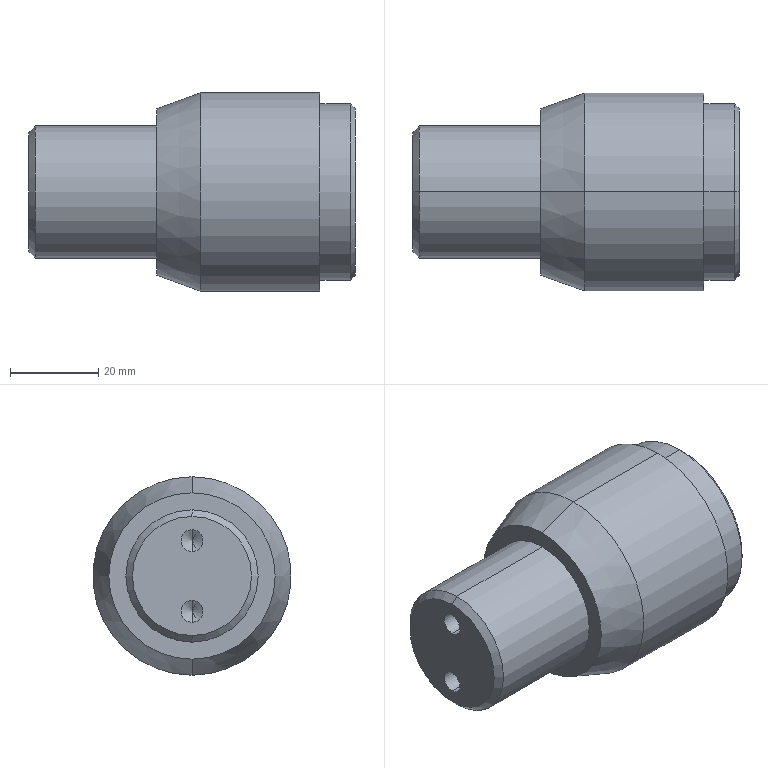Part | SolidWorks | features BaseBody 1 | 1 solid | 24 faces | box 74 x 45 x 45 mm | volume 86191 mm3 | cone 10 | cylinder 10 | plane 4 | commonest cylinder face diameters 5 x4 30 x2 40 x2 45 x2
STEP:
#1=CARTESIAN_POINT('',(-45.,0.,18.86));
#2=VERTEX_POINT('',#1);
#3=CARTESIAN_POINT('',(-45.,0.,-18.86));
#4=VERTEX_POINT('',#3);
#5=CARTESIAN_POINT('',(-45.,0.,0.));
#6=DIRECTION('',(-1.,0.,0.));
#7=DIRECTION('',(0.,0.,-1.));
#8=AXIS2_PLACEMENT_3D('',#5,#6,#7);
#9=CIRCLE('',#8,18.86);
#10=EDGE_CURVE('',#2,#4,#9,.T.);
#11=ORIENTED_EDGE('',*,*,#10,.F.);
#12=CARTESIAN_POINT('',(-35.,0.,22.5));
#13=VERTEX_POINT('',#12);
#14=CARTESIAN_POINT('',(-45.,0.,18.86));
#15=DIRECTION('',(0.9397,0.,0.342));
#16=VECTOR('',#15,1000.);
#17=LINE('',#14,#16);
#18=EDGE_CURVE('',#2,#13,#17,.T.);
#19=ORIENTED_EDGE('',*,*,#18,.T.);
#20=CARTESIAN_POINT('',(-35.,0.,-22.5));
#21=VERTEX_POINT('',#20);
#22=CARTESIAN_POINT('',(-35.,0.,0.));
#23=DIRECTION('',(1.,0.,0.));
#24=DIRECTION('',(0.,0.,-1.));
#25=AXIS2_PLACEMENT_3D('',#22,#23,#24);
#26=CIRCLE('',#25,22.5);
#27=EDGE_CURVE('',#21,#13,#26,.T.);
#28=ORIENTED_EDGE('',*,*,#27,.F.);
#29=CARTESIAN_POINT('',(-45.,0.,-18.86));
#30=DIRECTION('',(0.9397,0.,-0.342));
#31=VECTOR('',#30,1000.);
#32=LINE('',#29,#31);
#33=EDGE_CURVE('',#4,#21,#32,.T.);
#34=ORIENTED_EDGE('',*,*,#33,.F.);
#35=EDGE_LOOP('',(#11,#19,#28,#34));
#36=FACE_OUTER_BOUND('',#35,.T.);
#37=CARTESIAN_POINT('',(-45.,0.,0.));
#38=DIRECTION('',(1.,0.,0.));
#39=DIRECTION('',(0.,0.,-1.));
#40=AXIS2_PLACEMENT_3D('',#37,#38,#39);
#41=CONICAL_SURFACE('',#40,18.86,0.3491);
#42=ADVANCED_FACE('',(#36),#41,.T.);
#43=CARTESIAN_POINT('',(-59.,0.,-10.5));
#44=VERTEX_POINT('',#43);
#45=CARTESIAN_POINT('',(-59.,0.,-5.5));
#46=VERTEX_POINT('',#45);
#47=CARTESIAN_POINT('',(-59.,0.,-8.));
#48=DIRECTION('',(-1.,0.,0.));
#49=DIRECTION('',(0.,0.,1.));
#50=AXIS2_PLACEMENT_3D('',#47,#48,#49);
#51=CIRCLE('',#50,2.5);
#52=EDGE_CURVE('',#44,#46,#51,.T.);
#53=ORIENTED_EDGE('',*,*,#52,.F.);
#54=CARTESIAN_POINT('',(-74.,0.,-10.5));
#55=VERTEX_POINT('',#54);
#56=CARTESIAN_POINT('',(-74.,0.,-10.5));
#57=DIRECTION('',(-1.,0.,0.));
#58=VECTOR('',#57,1000.);
#59=LINE('',#56,#58);
#60=EDGE_CURVE('',#44,#55,#59,.T.);
#61=ORIENTED_EDGE('',*,*,#60,.T.);
#62=CARTESIAN_POINT('',(-74.,0.,-5.5));
#63=VERTEX_POINT('',#62);
#64=CARTESIAN_POINT('',(-74.,0.,-8.));
#65=DIRECTION('',(-1.,0.,0.));
#66=DIRECTION('',(0.,0.,1.));
#67=AXIS2_PLACEMENT_3D('',#64,#65,#66);
#68=CIRCLE('',#67,2.5);
#69=EDGE_CURVE('',#55,#63,#68,.T.);
#70=ORIENTED_EDGE('',*,*,#69,.T.);
#71=CARTESIAN_POINT('',(-74.,0.,-5.5));
#72=DIRECTION('',(-1.,0.,0.));
#73=VECTOR('',#72,1000.);
#74=LINE('',#71,#73);
#75=EDGE_CURVE('',#46,#63,#74,.T.);
#76=ORIENTED_EDGE('',*,*,#75,.F.);
#77=EDGE_LOOP('',(#53,#61,#70,#76));
#78=FACE_OUTER_BOUND('',#77,.T.);
#79=CARTESIAN_POINT('',(-74.,0.,-8.));
#80=DIRECTION('',(-1.,0.,0.));
#81=DIRECTION('',(0.,0.,1.));
#82=AXIS2_PLACEMENT_3D('',#79,#80,#81);
#83=CYLINDRICAL_SURFACE('',#82,2.5);
#84=ADVANCED_FACE('',(#78),#83,.F.);
#85=CARTESIAN_POINT('',(-57.498,0.,-8.));
#86=VERTEX_POINT('',#85);
#87=CARTESIAN_POINT('',(-59.,0.,-5.5));
#88=DIRECTION('',(-0.515,0.,0.8572));
#89=VECTOR('',#88,1000.);
#90=LINE('',#87,#89);
#91=EDGE_CURVE('',#86,#46,#90,.T.);
#92=ORIENTED_EDGE('',*,*,#91,.F.);
#93=CARTESIAN_POINT('',(-59.,0.,-10.5));
#94=DIRECTION('',(-0.515,0.,-0.8572));
#95=VECTOR('',#94,1000.);
#96=LINE('',#93,#95);
#97=EDGE_CURVE('',#86,#44,#96,.T.);
#98=ORIENTED_EDGE('',*,*,#97,.T.);
#99=ORIENTED_EDGE('',*,*,#52,.T.);
#100=EDGE_LOOP('',(#92,#98,#99));
#101=FACE_OUTER_BOUND('',#100,.T.);
#102=CARTESIAN_POINT('',(-59.,0.,-8.));
#103=DIRECTION('',(-1.,0.,0.));
#104=DIRECTION('',(0.,0.,1.));
#105=AXIS2_PLACEMENT_3D('',#102,#103,#104);
#106=CONICAL_SURFACE('',#105,2.5,1.03);
#107=ADVANCED_FACE('',(#101),#106,.F.);
#108=CARTESIAN_POINT('',(-59.,0.,5.5));
#109=VERTEX_POINT('',#108);
#110=CARTESIAN_POINT('',(-59.,0.,10.5));
#111=VERTEX_POINT('',#110);
#112=CARTESIAN_POINT('',(-59.,0.,8.));
#113=DIRECTION('',(-1.,0.,0.));
#114=DIRECTION('',(0.,0.,1.));
#115=AXIS2_PLACEMENT_3D('',#112,#113,#114);
#116=CIRCLE('',#115,2.5);
#117=EDGE_CURVE('',#109,#111,#116,.T.);
#118=ORIENTED_EDGE('',*,*,#117,.F.);
#119=CARTESIAN_POINT('',(-74.,0.,5.5));
#120=VERTEX_POINT('',#119);
#121=CARTESIAN_POINT('',(-74.,0.,5.5));
#122=DIRECTION('',(-1.,0.,0.));
#123=VECTOR('',#122,1000.);
#124=LINE('',#121,#123);
#125=EDGE_CURVE('',#109,#120,#124,.T.);
#126=ORIENTED_EDGE('',*,*,#125,.T.);
#127=CARTESIAN_POINT('',(-74.,0.,10.5));
#128=VERTEX_POINT('',#127);
#129=CARTESIAN_POINT('',(-74.,0.,8.));
#130=DIRECTION('',(-1.,0.,0.));
#131=DIRECTION('',(0.,0.,1.));
#132=AXIS2_PLACEMENT_3D('',#129,#130,#131);
#133=CIRCLE('',#132,2.5);
#134=EDGE_CURVE('',#120,#128,#133,.T.);
#135=ORIENTED_EDGE('',*,*,#134,.T.);
#136=CARTESIAN_POINT('',(-74.,0.,10.5));
#137=DIRECTION('',(-1.,0.,0.));
#138=VECTOR('',#137,1000.);
#139=LINE('',#136,#138);
#140=EDGE_CURVE('',#111,#128,#139,.T.);
#141=ORIENTED_EDGE('',*,*,#140,.F.);
#142=EDGE_LOOP('',(#118,#126,#135,#141));
#143=FACE_OUTER_BOUND('',#142,.T.);
#144=CARTESIAN_POINT('',(-74.,0.,8.));
#145=DIRECTION('',(-1.,0.,0.));
#146=DIRECTION('',(0.,0.,1.));
#147=AXIS2_PLACEMENT_3D('',#144,#145,#146);
#148=CYLINDRICAL_SURFACE('',#147,2.5);
#149=ADVANCED_FACE('',(#143),#148,.F.);
#150=CARTESIAN_POINT('',(-57.498,0.,8.));
#151=VERTEX_POINT('',#150);
#152=CARTESIAN_POINT('',(-59.,0.,10.5));
#153=DIRECTION('',(-0.515,0.,0.8572));
#154=VECTOR('',#153,1000.);
#155=LINE('',#152,#154);
#156=EDGE_CURVE('',#151,#111,#155,.T.);
#157=ORIENTED_EDGE('',*,*,#156,.F.);
#158=CARTESIAN_POINT('',(-59.,0.,5.5));
#159=DIRECTION('',(-0.515,0.,-0.8572));
#160=VECTOR('',#159,1000.);
#161=LINE('',#158,#160);
#162=EDGE_CURVE('',#151,#109,#161,.T.);
#163=ORIENTED_EDGE('',*,*,#162,.T.);
#164=ORIENTED_EDGE('',*,*,#117,.T.);
#165=EDGE_LOOP('',(#157,#163,#164));
#166=FACE_OUTER_BOUND('',#165,.T.);
#167=CARTESIAN_POINT('',(-59.,0.,8.));
#168=DIRECTION('',(-1.,0.,0.));
#169=DIRECTION('',(0.,0.,1.));
#170=AXIS2_PLACEMENT_3D('',#167,#168,#169);
#171=CONICAL_SURFACE('',#170,2.5,1.03);
#172=ADVANCED_FACE('',(#166),#171,.F.);
#173=CARTESIAN_POINT('',(-74.,0.,13.5));
#174=VERTEX_POINT('',#173);
#175=CARTESIAN_POINT('',(-74.,0.,-13.5));
#176=VERTEX_POINT('',#175);
#177=CARTESIAN_POINT('',(-74.,0.,0.));
#178=DIRECTION('',(-1.,0.,0.));
#179=DIRECTION('',(0.,0.,-1.));
#180=AXIS2_PLACEMENT_3D('',#177,#178,#179);
#181=CIRCLE('',#180,13.5);
#182=EDGE_CURVE('',#174,#176,#181,.T.);
#183=ORIENTED_EDGE('',*,*,#182,.F.);
#184=CARTESIAN_POINT('',(-72.5,0.,15.));
#185=VERTEX_POINT('',#184);
#186=CARTESIAN_POINT('',(-74.,0.,13.5));
#187=DIRECTION('',(0.7071,0.,0.7071));
#188=VECTOR('',#187,1000.);
#189=LINE('',#186,#188);
#190=EDGE_CURVE('',#174,#185,#189,.T.);
#191=ORIENTED_EDGE('',*,*,#190,.T.);
#192=CARTESIAN_POINT('',(-72.5,0.,-15.));
#193=VERTEX_POINT('',#192);
#194=CARTESIAN_POINT('',(-72.5,0.,0.));
#195=DIRECTION('',(1.,0.,0.));
#196=DIRECTION('',(0.,0.,-1.));
#197=AXIS2_PLACEMENT_3D('',#194,#195,#196);
#198=CIRCLE('',#197,15.);
#199=EDGE_CURVE('',#193,#185,#198,.T.);
#200=ORIENTED_EDGE('',*,*,#199,.F.);
#201=CARTESIAN_POINT('',(-74.,0.,-13.5));
#202=DIRECTION('',(0.7071,0.,-0.7071));
#203=VECTOR('',#202,1000.);
#204=LINE('',#201,#203);
#205=EDGE_CURVE('',#176,#193,#204,.T.);
#206=ORIENTED_EDGE('',*,*,#205,.F.);
#207=EDGE_LOOP('',(#183,#191,#200,#206));
#208=FACE_OUTER_BOUND('',#207,.T.);
#209=CARTESIAN_POINT('',(-74.,0.,0.));
#210=DIRECTION('',(1.,0.,0.));
#211=DIRECTION('',(0.,0.,-1.));
#212=AXIS2_PLACEMENT_3D('',#209,#210,#211);
#213=CONICAL_SURFACE('',#212,13.5,0.7854);
#214=ADVANCED_FACE('',(#208),#213,.T.);
#215=CARTESIAN_POINT('',(0.,0.,-19.));
#216=VERTEX_POINT('',#215);
#217=CARTESIAN_POINT('',(0.,0.,19.));
#218=VERTEX_POINT('',#217);
#219=CARTESIAN_POINT('',(0.,0.,0.));
#220=DIRECTION('',(1.,0.,0.));
#221=DIRECTION('',(0.,0.,1.));
#222=AXIS2_PLACEMENT_3D('',#219,#220,#221);
#223=CIRCLE('',#222,19.);
#224=EDGE_CURVE('',#216,#218,#223,.T.);
#225=ORIENTED_EDGE('',*,*,#224,.F.);
#226=CARTESIAN_POINT('',(-1.,0.,-20.));
#227=VERTEX_POINT('',#226);
#228=CARTESIAN_POINT('',(-1.,0.,-20.));
#229=DIRECTION('',(-0.7071,0.,-0.7071));
#230=VECTOR('',#229,1000.);
#231=LINE('',#228,#230);
#232=EDGE_CURVE('',#216,#227,#231,.T.);
#233=ORIENTED_EDGE('',*,*,#232,.T.);
#234=CARTESIAN_POINT('',(-1.,0.,20.));
#235=VERTEX_POINT('',#234);
#236=CARTESIAN_POINT('',(-1.,0.,0.));
#237=DIRECTION('',(-1.,0.,0.));
#238=DIRECTION('',(0.,0.,1.));
#239=AXIS2_PLACEMENT_3D('',#236,#237,#238);
#240=CIRCLE('',#239,20.);
#241=EDGE_CURVE('',#235,#227,#240,.T.);
#242=ORIENTED_EDGE('',*,*,#241,.F.);
#243=CARTESIAN_POINT('',(-1.,0.,20.));
#244=DIRECTION('',(-0.7071,0.,0.7071));
#245=VECTOR('',#244,1000.);
#246=LINE('',#243,#245);
#247=EDGE_CURVE('',#218,#235,#246,.T.);
#248=ORIENTED_EDGE('',*,*,#247,.F.);
#249=EDGE_LOOP('',(#225,#233,#242,#248));
#250=FACE_OUTER_BOUND('',#249,.T.);
#251=CARTESIAN_POINT('',(-1.,0.,0.));
#252=DIRECTION('',(-1.,0.,0.));
#253=DIRECTION('',(0.,0.,1.));
#254=AXIS2_PLACEMENT_3D('',#251,#252,#253);
#255=CONICAL_SURFACE('',#254,20.,0.7854);
#256=ADVANCED_FACE('',(#250),#255,.T.);
#257=CARTESIAN_POINT('',(-45.,0.,15.));
#258=VERTEX_POINT('',#257);
#259=CARTESIAN_POINT('',(-45.,0.,-15.));
#260=VERTEX_POINT('',#259);
#261=CARTESIAN_POINT('',(-45.,0.,0.));
#262=DIRECTION('',(-1.,0.,0.));
#263=DIRECTION('',(0.,0.,1.));
#264=AXIS2_PLACEMENT_3D('',#261,#262,#263);
#265=CIRCLE('',#264,15.);
#266=EDGE_CURVE('',#258,#260,#265,.T.);
#267=ORIENTED_EDGE('',*,*,#266,.T.);
#268=CARTESIAN_POINT('',(-74.,0.,-15.));
#269=DIRECTION('',(-1.,0.,0.));
#270=VECTOR('',#269,1000.);
#271=LINE('',#268,#270);
#272=EDGE_CURVE('',#260,#193,#271,.T.);
#273=ORIENTED_EDGE('',*,*,#272,.T.);
#274=ORIENTED_EDGE('',*,*,#199,.T.);
#275=CARTESIAN_POINT('',(-74.,0.,15.));
#276=DIRECTION('',(-1.,0.,0.));
#277=VECTOR('',#276,1000.);
#278=LINE('',#275,#277);
#279=EDGE_CURVE('',#258,#185,#278,.T.);
#280=ORIENTED_EDGE('',*,*,#279,.F.);
#281=EDGE_LOOP('',(#267,#273,#274,#280));
#282=FACE_OUTER_BOUND('',#281,.T.);
#283=CARTESIAN_POINT('',(-74.,0.,0.));
#284=DIRECTION('',(-1.,0.,0.));
#285=DIRECTION('',(0.,0.,1.));
#286=AXIS2_PLACEMENT_3D('',#283,#284,#285);
#287=CYLINDRICAL_SURFACE('',#286,15.);
#288=ADVANCED_FACE('',(#282),#287,.T.);
#289=CARTESIAN_POINT('',(-8.,0.,22.5));
#290=VERTEX_POINT('',#289);
#291=CARTESIAN_POINT('',(-8.,0.,-22.5));
#292=VERTEX_POINT('',#291);
#293=CARTESIAN_POINT('',(-8.,0.,0.));
#294=DIRECTION('',(-1.,0.,0.));
#295=DIRECTION('',(0.,0.,1.));
#296=AXIS2_PLACEMENT_3D('',#293,#294,#295);
#297=CIRCLE('',#296,22.5);
#298=EDGE_CURVE('',#290,#292,#297,.T.);
#299=ORIENTED_EDGE('',*,*,#298,.T.);
#300=CARTESIAN_POINT('',(-74.,0.,-22.5));
#301=DIRECTION('',(-1.,0.,0.));
#302=VECTOR('',#301,1000.);
#303=LINE('',#300,#302);
#304=EDGE_CURVE('',#292,#21,#303,.T.);
#305=ORIENTED_EDGE('',*,*,#304,.T.);
#306=ORIENTED_EDGE('',*,*,#27,.T.);
#307=CARTESIAN_POINT('',(-74.,0.,22.5));
#308=DIRECTION('',(-1.,0.,0.));
#309=VECTOR('',#308,1000.);
#310=LINE('',#307,#309);
#311=EDGE_CURVE('',#290,#13,#310,.T.);
#312=ORIENTED_EDGE('',*,*,#311,.F.);
#313=EDGE_LOOP('',(#299,#305,#306,#312));
#314=FACE_OUTER_BOUND('',#313,.T.);
#315=CARTESIAN_POINT('',(-74.,0.,0.));
#316=DIRECTION('',(-1.,0.,0.));
#317=DIRECTION('',(0.,0.,1.));
#318=AXIS2_PLACEMENT_3D('',#315,#316,#317);
#319=CYLINDRICAL_SURFACE('',#318,22.5);
#320=ADVANCED_FACE('',(#314),#319,.T.);
#321=ORIENTED_EDGE('',*,*,#241,.T.);
#322=CARTESIAN_POINT('',(-8.,0.,-20.));
#323=VERTEX_POINT('',#322);
#324=CARTESIAN_POINT('',(-74.,0.,-20.));
#325=DIRECTION('',(-1.,0.,0.));
#326=VECTOR('',#325,1000.);
#327=LINE('',#324,#326);
#328=EDGE_CURVE('',#227,#323,#327,.T.);
#329=ORIENTED_EDGE('',*,*,#328,.T.);
#330=CARTESIAN_POINT('',(-8.,0.,20.));
#331=VERTEX_POINT('',#330);
#332=CARTESIAN_POINT('',(-8.,0.,0.));
#333=DIRECTION('',(-1.,0.,0.));
#334=DIRECTION('',(0.,0.,1.));
#335=AXIS2_PLACEMENT_3D('',#332,#333,#334);
#336=CIRCLE('',#335,20.);
#337=EDGE_CURVE('',#331,#323,#336,.T.);
#338=ORIENTED_EDGE('',*,*,#337,.F.);
#339=CARTESIAN_POINT('',(-74.,0.,20.));
#340=DIRECTION('',(-1.,0.,0.));
#341=VECTOR('',#340,1000.);
#342=LINE('',#339,#341);
#343=EDGE_CURVE('',#235,#331,#342,.T.);
#344=ORIENTED_EDGE('',*,*,#343,.F.);
#345=EDGE_LOOP('',(#321,#329,#338,#344));
#346=FACE_OUTER_BOUND('',#345,.T.);
#347=CARTESIAN_POINT('',(-74.,0.,0.));
#348=DIRECTION('',(-1.,0.,0.));
#349=DIRECTION('',(0.,0.,1.));
#350=AXIS2_PLACEMENT_3D('',#347,#348,#349);
#351=CYLINDRICAL_SURFACE('',#350,20.);
#352=ADVANCED_FACE('',(#346),#351,.T.);
#353=CARTESIAN_POINT('',(-74.,0.,8.));
#354=DIRECTION('',(-1.,0.,0.));
#355=DIRECTION('',(0.,0.,1.));
#356=AXIS2_PLACEMENT_3D('',#353,#354,#355);
#357=CIRCLE('',#356,2.5);
#358=EDGE_CURVE('',#128,#120,#357,.T.);
#359=ORIENTED_EDGE('',*,*,#358,.F.);
#360=ORIENTED_EDGE('',*,*,#134,.F.);
#361=EDGE_LOOP('',(#359,#360));
#362=FACE_BOUND('',#361,.T.);
#363=CARTESIAN_POINT('',(-74.,0.,-8.));
#364=DIRECTION('',(-1.,0.,0.));
#365=DIRECTION('',(0.,0.,1.));
#366=AXIS2_PLACEMENT_3D('',#363,#364,#365);
#367=CIRCLE('',#366,2.5);
#368=EDGE_CURVE('',#63,#55,#367,.T.);
#369=ORIENTED_EDGE('',*,*,#368,.F.);
#370=ORIENTED_EDGE('',*,*,#69,.F.);
#371=EDGE_LOOP('',(#369,#370));
#372=FACE_BOUND('',#371,.T.);
#373=CARTESIAN_POINT('',(-74.,0.,0.));
#374=DIRECTION('',(-1.,0.,0.));
#375=DIRECTION('',(0.,0.,-1.));
#376=AXIS2_PLACEMENT_3D('',#373,#374,#375);
#377=CIRCLE('',#376,13.5);
#378=EDGE_CURVE('',#176,#174,#377,.T.);
#379=ORIENTED_EDGE('',*,*,#378,.T.);
#380=ORIENTED_EDGE('',*,*,#182,.T.);
#381=EDGE_LOOP('',(#379,#380));
#382=FACE_OUTER_BOUND('',#381,.T.);
#383=CARTESIAN_POINT('',(-74.,15.,0.));
#384=DIRECTION('',(1.,0.,0.));
#385=DIRECTION('',(0.,1.,0.));
#386=AXIS2_PLACEMENT_3D('',#383,#384,#385);
#387=PLANE('',#386);
#388=ADVANCED_FACE('',(#362,#372,#382),#387,.F.);
#389=ORIENTED_EDGE('',*,*,#266,.F.);
#390=CARTESIAN_POINT('',(-45.,0.,0.));
#391=DIRECTION('',(-1.,0.,0.));
#392=DIRECTION('',(0.,0.,1.));
#393=AXIS2_PLACEMENT_3D('',#390,#391,#392);
#394=CIRCLE('',#393,15.);
#395=EDGE_CURVE('',#260,#258,#394,.T.);
#396=ORIENTED_EDGE('',*,*,#395,.F.);
#397=EDGE_LOOP('',(#389,#396));
#398=FACE_BOUND('',#397,.T.);
#399=CARTESIAN_POINT('',(-45.,0.,0.));
#400=DIRECTION('',(-1.,0.,0.));
#401=DIRECTION('',(0.,0.,-1.));
#402=AXIS2_PLACEMENT_3D('',#399,#400,#401);
#403=CIRCLE('',#402,18.86);
#404=EDGE_CURVE('',#4,#2,#403,.T.);
#405=ORIENTED_EDGE('',*,*,#404,.T.);
#406=ORIENTED_EDGE('',*,*,#10,.T.);
#407=EDGE_LOOP('',(#405,#406));
#408=FACE_OUTER_BOUND('',#407,.T.);
#409=CARTESIAN_POINT('',(-45.,22.5,0.));
#410=DIRECTION('',(1.,0.,0.));
#411=DIRECTION('',(0.,1.,0.));
#412=AXIS2_PLACEMENT_3D('',#409,#410,#411);
#413=PLANE('',#412);
#414=ADVANCED_FACE('',(#398,#408),#413,.F.);
#415=ORIENTED_EDGE('',*,*,#337,.T.);
#416=CARTESIAN_POINT('',(-8.,0.,0.));
#417=DIRECTION('',(-1.,0.,0.));
#418=DIRECTION('',(0.,0.,1.));
#419=AXIS2_PLACEMENT_3D('',#416,#417,#418);
#420=CIRCLE('',#419,20.);
#421=EDGE_CURVE('',#323,#331,#420,.T.);
#422=ORIENTED_EDGE('',*,*,#421,.T.);
#423=EDGE_LOOP('',(#415,#422));
#424=FACE_BOUND('',#423,.T.);
#425=ORIENTED_EDGE('',*,*,#298,.F.);
#426=CARTESIAN_POINT('',(-8.,0.,0.));
#427=DIRECTION('',(-1.,0.,0.));
#428=DIRECTION('',(0.,0.,1.));
#429=AXIS2_PLACEMENT_3D('',#426,#427,#428);
#430=CIRCLE('',#429,22.5);
#431=EDGE_CURVE('',#292,#290,#430,.T.);
#432=ORIENTED_EDGE('',*,*,#431,.F.);
#433=EDGE_LOOP('',(#425,#432));
#434=FACE_OUTER_BOUND('',#433,.T.);
#435=CARTESIAN_POINT('',(-8.,20.,0.));
#436=DIRECTION('',(-1.,0.,0.));
#437=DIRECTION('',(0.,0.,1.));
#438=AXIS2_PLACEMENT_3D('',#435,#436,#437);
#439=PLANE('',#438);
#440=ADVANCED_FACE('',(#424,#434),#439,.F.);
#441=CARTESIAN_POINT('',(0.,0.,0.));
#442=DIRECTION('',(1.,0.,0.));
#443=DIRECTION('',(0.,0.,1.));
#444=AXIS2_PLACEMENT_3D('',#441,#442,#443);
#445=CIRCLE('',#444,19.);
#446=EDGE_CURVE('',#218,#216,#445,.T.);
#447=ORIENTED_EDGE('',*,*,#446,.T.);
#448=ORIENTED_EDGE('',*,*,#224,.T.);
#449=EDGE_LOOP('',(#447,#448));
#450=FACE_OUTER_BOUND('',#449,.T.);
#451=CARTESIAN_POINT('',(0.,0.,0.));
#452=DIRECTION('',(-1.,0.,0.));
#453=DIRECTION('',(0.,0.,1.));
#454=AXIS2_PLACEMENT_3D('',#451,#452,#453);
#455=PLANE('',#454);
#456=ADVANCED_FACE('',(#450),#455,.F.);
#457=ORIENTED_EDGE('',*,*,#328,.F.);
#458=CARTESIAN_POINT('',(-1.,0.,0.));
#459=DIRECTION('',(-1.,0.,0.));
#460=DIRECTION('',(0.,0.,1.));
#461=AXIS2_PLACEMENT_3D('',#458,#459,#460);
#462=CIRCLE('',#461,20.);
#463=EDGE_CURVE('',#227,#235,#462,.T.);
#464=ORIENTED_EDGE('',*,*,#463,.T.);
#465=ORIENTED_EDGE('',*,*,#343,.T.);
#466=ORIENTED_EDGE('',*,*,#421,.F.);
#467=EDGE_LOOP('',(#457,#464,#465,#466));
#468=FACE_OUTER_BOUND('',#467,.T.);
#469=CARTESIAN_POINT('',(-74.,0.,0.));
#470=DIRECTION('',(-1.,0.,0.));
#471=DIRECTION('',(0.,0.,1.));
#472=AXIS2_PLACEMENT_3D('',#469,#470,#471);
#473=CYLINDRICAL_SURFACE('',#472,20.);
#474=ADVANCED_FACE('',(#468),#473,.T.);
#475=ORIENTED_EDGE('',*,*,#304,.F.);
#476=ORIENTED_EDGE('',*,*,#431,.T.);
#477=ORIENTED_EDGE('',*,*,#311,.T.);
#478=CARTESIAN_POINT('',(-35.,0.,0.));
#479=DIRECTION('',(1.,0.,0.));
#480=DIRECTION('',(0.,0.,-1.));
#481=AXIS2_PLACEMENT_3D('',#478,#479,#480);
#482=CIRCLE('',#481,22.5);
#483=EDGE_CURVE('',#13,#21,#482,.T.);
#484=ORIENTED_EDGE('',*,*,#483,.T.);
#485=EDGE_LOOP('',(#475,#476,#477,#484));
#486=FACE_OUTER_BOUND('',#485,.T.);
#487=CARTESIAN_POINT('',(-74.,0.,0.));
#488=DIRECTION('',(-1.,0.,0.));
#489=DIRECTION('',(0.,0.,1.));
#490=AXIS2_PLACEMENT_3D('',#487,#488,#489);
#491=CYLINDRICAL_SURFACE('',#490,22.5);
#492=ADVANCED_FACE('',(#486),#491,.T.);
#493=ORIENTED_EDGE('',*,*,#272,.F.);
#494=ORIENTED_EDGE('',*,*,#395,.T.);
#495=ORIENTED_EDGE('',*,*,#279,.T.);
#496=CARTESIAN_POINT('',(-72.5,0.,0.));
#497=DIRECTION('',(1.,0.,0.));
#498=DIRECTION('',(0.,0.,-1.));
#499=AXIS2_PLACEMENT_3D('',#496,#497,#498);
#500=CIRCLE('',#499,15.);
#501=EDGE_CURVE('',#185,#193,#500,.T.);
#502=ORIENTED_EDGE('',*,*,#501,.T.);
#503=EDGE_LOOP('',(#493,#494,#495,#502));
#504=FACE_OUTER_BOUND('',#503,.T.);
#505=CARTESIAN_POINT('',(-74.,0.,0.));
#506=DIRECTION('',(-1.,0.,0.));
#507=DIRECTION('',(0.,0.,1.));
#508=AXIS2_PLACEMENT_3D('',#505,#506,#507);
#509=CYLINDRICAL_SURFACE('',#508,15.);
#510=ADVANCED_FACE('',(#504),#509,.T.);
#511=ORIENTED_EDGE('',*,*,#232,.F.);
#512=ORIENTED_EDGE('',*,*,#446,.F.);
#513=ORIENTED_EDGE('',*,*,#247,.T.);
#514=ORIENTED_EDGE('',*,*,#463,.F.);
#515=EDGE_LOOP('',(#511,#512,#513,#514));
#516=FACE_OUTER_BOUND('',#515,.T.);
#517=CARTESIAN_POINT('',(-1.,0.,0.));
#518=DIRECTION('',(-1.,0.,0.));
#519=DIRECTION('',(0.,0.,1.));
#520=AXIS2_PLACEMENT_3D('',#517,#518,#519);
#521=CONICAL_SURFACE('',#520,20.,0.7854);
#522=ADVANCED_FACE('',(#516),#521,.T.);
#523=ORIENTED_EDGE('',*,*,#190,.F.);
#524=ORIENTED_EDGE('',*,*,#378,.F.);
#525=ORIENTED_EDGE('',*,*,#205,.T.);
#526=ORIENTED_EDGE('',*,*,#501,.F.);
#527=EDGE_LOOP('',(#523,#524,#525,#526));
#528=FACE_OUTER_BOUND('',#527,.T.);
#529=CARTESIAN_POINT('',(-74.,0.,0.));
#530=DIRECTION('',(1.,0.,0.));
#531=DIRECTION('',(0.,0.,-1.));
#532=AXIS2_PLACEMENT_3D('',#529,#530,#531);
#533=CONICAL_SURFACE('',#532,13.5,0.7854);
#534=ADVANCED_FACE('',(#528),#533,.T.);
#535=ORIENTED_EDGE('',*,*,#162,.F.);
#536=ORIENTED_EDGE('',*,*,#156,.T.);
#537=CARTESIAN_POINT('',(-59.,0.,8.));
#538=DIRECTION('',(-1.,0.,0.));
#539=DIRECTION('',(0.,0.,1.));
#540=AXIS2_PLACEMENT_3D('',#537,#538,#539);
#541=CIRCLE('',#540,2.5);
#542=EDGE_CURVE('',#111,#109,#541,.T.);
#543=ORIENTED_EDGE('',*,*,#542,.T.);
#544=EDGE_LOOP('',(#535,#536,#543));
#545=FACE_OUTER_BOUND('',#544,.T.);
#546=CARTESIAN_POINT('',(-59.,0.,8.));
#547=DIRECTION('',(-1.,0.,0.));
#548=DIRECTION('',(0.,0.,1.));
#549=AXIS2_PLACEMENT_3D('',#546,#547,#548);
#550=CONICAL_SURFACE('',#549,2.5,1.03);
#551=ADVANCED_FACE('',(#545),#550,.F.);
#552=ORIENTED_EDGE('',*,*,#125,.F.);
#553=ORIENTED_EDGE('',*,*,#542,.F.);
#554=ORIENTED_EDGE('',*,*,#140,.T.);
#555=ORIENTED_EDGE('',*,*,#358,.T.);
#556=EDGE_LOOP('',(#552,#553,#554,#555));
#557=FACE_OUTER_BOUND('',#556,.T.);
#558=CARTESIAN_POINT('',(-74.,0.,8.));
#559=DIRECTION('',(-1.,0.,0.));
#560=DIRECTION('',(0.,0.,1.));
#561=AXIS2_PLACEMENT_3D('',#558,#559,#560);
#562=CYLINDRICAL_SURFACE('',#561,2.5);
#563=ADVANCED_FACE('',(#557),#562,.F.);
#564=ORIENTED_EDGE('',*,*,#97,.F.);
#565=ORIENTED_EDGE('',*,*,#91,.T.);
#566=CARTESIAN_POINT('',(-59.,0.,-8.));
#567=DIRECTION('',(-1.,0.,0.));
#568=DIRECTION('',(0.,0.,1.));
#569=AXIS2_PLACEMENT_3D('',#566,#567,#568);
#570=CIRCLE('',#569,2.5);
#571=EDGE_CURVE('',#46,#44,#570,.T.);
#572=ORIENTED_EDGE('',*,*,#571,.T.);
#573=EDGE_LOOP('',(#564,#565,#572));
#574=FACE_OUTER_BOUND('',#573,.T.);
#575=CARTESIAN_POINT('',(-59.,0.,-8.));
#576=DIRECTION('',(-1.,0.,0.));
#577=DIRECTION('',(0.,0.,1.));
#578=AXIS2_PLACEMENT_3D('',#575,#576,#577);
#579=CONICAL_SURFACE('',#578,2.5,1.03);
#580=ADVANCED_FACE('',(#574),#579,.F.);
#581=ORIENTED_EDGE('',*,*,#60,.F.);
#582=ORIENTED_EDGE('',*,*,#571,.F.);
#583=ORIENTED_EDGE('',*,*,#75,.T.);
#584=ORIENTED_EDGE('',*,*,#368,.T.);
#585=EDGE_LOOP('',(#581,#582,#583,#584));
#586=FACE_OUTER_BOUND('',#585,.T.);
#587=CARTESIAN_POINT('',(-74.,0.,-8.));
#588=DIRECTION('',(-1.,0.,0.));
#589=DIRECTION('',(0.,0.,1.));
#590=AXIS2_PLACEMENT_3D('',#587,#588,#589);
#591=CYLINDRICAL_SURFACE('',#590,2.5);
#592=ADVANCED_FACE('',(#586),#591,.F.);
#593=ORIENTED_EDGE('',*,*,#18,.F.);
#594=ORIENTED_EDGE('',*,*,#404,.F.);
#595=ORIENTED_EDGE('',*,*,#33,.T.);
#596=ORIENTED_EDGE('',*,*,#483,.F.);
#597=EDGE_LOOP('',(#593,#594,#595,#596));
#598=FACE_OUTER_BOUND('',#597,.T.);
#599=CARTESIAN_POINT('',(-45.,0.,0.));
#600=DIRECTION('',(1.,0.,0.));
#601=DIRECTION('',(0.,0.,-1.));
#602=AXIS2_PLACEMENT_3D('',#599,#600,#601);
#603=CONICAL_SURFACE('',#602,18.86,0.3491);
#604=ADVANCED_FACE('',(#598),#603,.T.);
#605=CLOSED_SHELL('',(#42,#84,#107,#149,#172,#214,#256,#288,#320,#352,#388,#414,#440,#456,#474,#492,#510,#522,#534,#551,#563,#580,#592,#604));
#606=MANIFOLD_SOLID_BREP('',#605);
#607=CARTESIAN_POINT('',(0.,0.,0.));
#608=DIRECTION('',(0.,0.,1.));
#609=DIRECTION('',(1.,0.,0.));
#610=AXIS2_PLACEMENT_3D('',#607,#608,#609);
#611=(LENGTH_UNIT()NAMED_UNIT(*)SI_UNIT(.MILLI.,.METRE.));
#612=UNCERTAINTY_MEASURE_WITH_UNIT(LENGTH_MEASURE(0.00001),#611,'','');
#613=(NAMED_UNIT(*)PLANE_ANGLE_UNIT()SI_UNIT($,.RADIAN.));
#614=(NAMED_UNIT(*)SI_UNIT($,.STERADIAN.)SOLID_ANGLE_UNIT());
#615=(GEOMETRIC_REPRESENTATION_CONTEXT(3)GLOBAL_UNCERTAINTY_ASSIGNED_CONTEXT((#612))GLOBAL_UNIT_ASSIGNED_CONTEXT((#611,#613,#614))REPRESENTATION_CONTEXT('',''));
#616=ADVANCED_BREP_SHAPE_REPRESENTATION('',(#606,#610),#615);